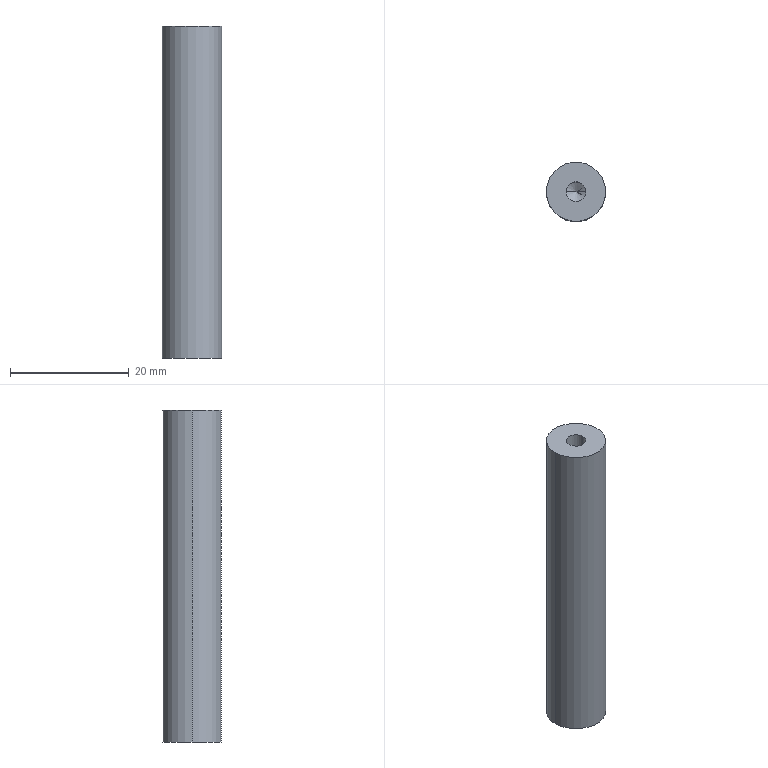Part | STEP file | 11-FG-Z00711 | 1 solid | 12 faces | box 10 x 10 x 56 mm | volume 4220 mm3 | cylinder 6 | cone 4 | plane 2 | commonest cylinder face diameters 3.3 x4 10 x2
STEP:
#1=CARTESIAN_POINT('',(1.65,0.,-45.9));
#2=VERTEX_POINT('',#1);
#3=CARTESIAN_POINT('',(-1.65,0.,-45.9));
#4=VERTEX_POINT('',#3);
#5=CARTESIAN_POINT('',(0.,0.,-45.9));
#6=DIRECTION('',(0.,0.,-1.));
#7=DIRECTION('',(-1.,0.,0.));
#8=AXIS2_PLACEMENT_3D('',#5,#6,#7);
#9=CIRCLE('',#8,1.65);
#10=EDGE_CURVE('',#2,#4,#9,.T.);
#11=ORIENTED_EDGE('',*,*,#10,.F.);
#12=CARTESIAN_POINT('',(1.65,0.,-56.));
#13=VERTEX_POINT('',#12);
#14=CARTESIAN_POINT('',(1.65,0.,-56.));
#15=DIRECTION('',(0.,0.,-1.));
#16=VECTOR('',#15,1000.);
#17=LINE('',#14,#16);
#18=EDGE_CURVE('',#2,#13,#17,.T.);
#19=ORIENTED_EDGE('',*,*,#18,.T.);
#20=CARTESIAN_POINT('',(-1.65,0.,-56.));
#21=VERTEX_POINT('',#20);
#22=CARTESIAN_POINT('',(0.,0.,-56.));
#23=DIRECTION('',(0.,0.,-1.));
#24=DIRECTION('',(-1.,0.,0.));
#25=AXIS2_PLACEMENT_3D('',#22,#23,#24);
#26=CIRCLE('',#25,1.65);
#27=EDGE_CURVE('',#13,#21,#26,.T.);
#28=ORIENTED_EDGE('',*,*,#27,.T.);
#29=CARTESIAN_POINT('',(-1.65,0.,-56.));
#30=DIRECTION('',(0.,0.,-1.));
#31=VECTOR('',#30,1000.);
#32=LINE('',#29,#31);
#33=EDGE_CURVE('',#4,#21,#32,.T.);
#34=ORIENTED_EDGE('',*,*,#33,.F.);
#35=EDGE_LOOP('',(#11,#19,#28,#34));
#36=FACE_OUTER_BOUND('',#35,.T.);
#37=CARTESIAN_POINT('',(0.,0.,-56.));
#38=DIRECTION('',(0.,0.,-1.));
#39=DIRECTION('',(-1.,0.,0.));
#40=AXIS2_PLACEMENT_3D('',#37,#38,#39);
#41=CYLINDRICAL_SURFACE('',#40,1.65);
#42=ADVANCED_FACE('',(#36),#41,.F.);
#43=CARTESIAN_POINT('',(0.,0.,-44.909));
#44=VERTEX_POINT('',#43);
#45=CARTESIAN_POINT('',(-1.65,0.,-45.9));
#46=DIRECTION('',(-0.8572,0.,-0.515));
#47=VECTOR('',#46,1000.);
#48=LINE('',#45,#47);
#49=EDGE_CURVE('',#44,#4,#48,.T.);
#50=ORIENTED_EDGE('',*,*,#49,.F.);
#51=CARTESIAN_POINT('',(1.65,0.,-45.9));
#52=DIRECTION('',(0.8572,0.,-0.515));
#53=VECTOR('',#52,1000.);
#54=LINE('',#51,#53);
#55=EDGE_CURVE('',#44,#2,#54,.T.);
#56=ORIENTED_EDGE('',*,*,#55,.T.);
#57=ORIENTED_EDGE('',*,*,#10,.T.);
#58=EDGE_LOOP('',(#50,#56,#57));
#59=FACE_OUTER_BOUND('',#58,.T.);
#60=CARTESIAN_POINT('',(0.,0.,-45.9));
#61=DIRECTION('',(0.,0.,-1.));
#62=DIRECTION('',(-1.,0.,0.));
#63=AXIS2_PLACEMENT_3D('',#60,#61,#62);
#64=CONICAL_SURFACE('',#63,1.65,1.03);
#65=ADVANCED_FACE('',(#59),#64,.F.);
#66=CARTESIAN_POINT('',(-1.65,0.,-10.1));
#67=VERTEX_POINT('',#66);
#68=CARTESIAN_POINT('',(1.65,0.,-10.1));
#69=VERTEX_POINT('',#68);
#70=CARTESIAN_POINT('',(0.,0.,-10.1));
#71=DIRECTION('',(0.,0.,1.));
#72=DIRECTION('',(1.,0.,0.));
#73=AXIS2_PLACEMENT_3D('',#70,#71,#72);
#74=CIRCLE('',#73,1.65);
#75=EDGE_CURVE('',#67,#69,#74,.T.);
#76=ORIENTED_EDGE('',*,*,#75,.F.);
#77=CARTESIAN_POINT('',(-1.65,0.,0.));
#78=VERTEX_POINT('',#77);
#79=CARTESIAN_POINT('',(-1.65,0.,0.));
#80=DIRECTION('',(0.,0.,1.));
#81=VECTOR('',#80,1000.);
#82=LINE('',#79,#81);
#83=EDGE_CURVE('',#67,#78,#82,.T.);
#84=ORIENTED_EDGE('',*,*,#83,.T.);
#85=CARTESIAN_POINT('',(1.65,0.,0.));
#86=VERTEX_POINT('',#85);
#87=CARTESIAN_POINT('',(0.,0.,0.));
#88=DIRECTION('',(0.,0.,1.));
#89=DIRECTION('',(1.,0.,0.));
#90=AXIS2_PLACEMENT_3D('',#87,#88,#89);
#91=CIRCLE('',#90,1.65);
#92=EDGE_CURVE('',#78,#86,#91,.T.);
#93=ORIENTED_EDGE('',*,*,#92,.T.);
#94=CARTESIAN_POINT('',(1.65,0.,0.));
#95=DIRECTION('',(0.,0.,1.));
#96=VECTOR('',#95,1000.);
#97=LINE('',#94,#96);
#98=EDGE_CURVE('',#69,#86,#97,.T.);
#99=ORIENTED_EDGE('',*,*,#98,.F.);
#100=EDGE_LOOP('',(#76,#84,#93,#99));
#101=FACE_OUTER_BOUND('',#100,.T.);
#102=CARTESIAN_POINT('',(0.,0.,0.));
#103=DIRECTION('',(0.,0.,1.));
#104=DIRECTION('',(1.,0.,0.));
#105=AXIS2_PLACEMENT_3D('',#102,#103,#104);
#106=CYLINDRICAL_SURFACE('',#105,1.65);
#107=ADVANCED_FACE('',(#101),#106,.F.);
#108=CARTESIAN_POINT('',(0.,0.,-11.091));
#109=VERTEX_POINT('',#108);
#110=CARTESIAN_POINT('',(1.65,0.,-10.1));
#111=DIRECTION('',(0.8572,0.,0.515));
#112=VECTOR('',#111,1000.);
#113=LINE('',#110,#112);
#114=EDGE_CURVE('',#109,#69,#113,.T.);
#115=ORIENTED_EDGE('',*,*,#114,.F.);
#116=CARTESIAN_POINT('',(-1.65,0.,-10.1));
#117=DIRECTION('',(-0.8572,0.,0.515));
#118=VECTOR('',#117,1000.);
#119=LINE('',#116,#118);
#120=EDGE_CURVE('',#109,#67,#119,.T.);
#121=ORIENTED_EDGE('',*,*,#120,.T.);
#122=ORIENTED_EDGE('',*,*,#75,.T.);
#123=EDGE_LOOP('',(#115,#121,#122));
#124=FACE_OUTER_BOUND('',#123,.T.);
#125=CARTESIAN_POINT('',(0.,0.,-10.1));
#126=DIRECTION('',(0.,0.,1.));
#127=DIRECTION('',(1.,0.,0.));
#128=AXIS2_PLACEMENT_3D('',#125,#126,#127);
#129=CONICAL_SURFACE('',#128,1.65,1.03);
#130=ADVANCED_FACE('',(#124),#129,.F.);
#131=CARTESIAN_POINT('',(5.,0.,-56.));
#132=VERTEX_POINT('',#131);
#133=CARTESIAN_POINT('',(-5.,0.,-56.));
#134=VERTEX_POINT('',#133);
#135=CARTESIAN_POINT('',(0.,0.,-56.));
#136=DIRECTION('',(0.,0.,1.));
#137=DIRECTION('',(1.,0.,0.));
#138=AXIS2_PLACEMENT_3D('',#135,#136,#137);
#139=CIRCLE('',#138,5.);
#140=EDGE_CURVE('',#132,#134,#139,.T.);
#141=ORIENTED_EDGE('',*,*,#140,.T.);
#142=CARTESIAN_POINT('',(-5.,0.,0.));
#143=VERTEX_POINT('',#142);
#144=CARTESIAN_POINT('',(-5.,0.,-56.));
#145=DIRECTION('',(0.,0.,1.));
#146=VECTOR('',#145,1000.);
#147=LINE('',#144,#146);
#148=EDGE_CURVE('',#134,#143,#147,.T.);
#149=ORIENTED_EDGE('',*,*,#148,.T.);
#150=CARTESIAN_POINT('',(5.,0.,0.));
#151=VERTEX_POINT('',#150);
#152=CARTESIAN_POINT('',(0.,0.,0.));
#153=DIRECTION('',(0.,0.,1.));
#154=DIRECTION('',(1.,0.,0.));
#155=AXIS2_PLACEMENT_3D('',#152,#153,#154);
#156=CIRCLE('',#155,5.);
#157=EDGE_CURVE('',#151,#143,#156,.T.);
#158=ORIENTED_EDGE('',*,*,#157,.F.);
#159=CARTESIAN_POINT('',(5.,0.,-56.));
#160=DIRECTION('',(0.,0.,1.));
#161=VECTOR('',#160,1000.);
#162=LINE('',#159,#161);
#163=EDGE_CURVE('',#132,#151,#162,.T.);
#164=ORIENTED_EDGE('',*,*,#163,.F.);
#165=EDGE_LOOP('',(#141,#149,#158,#164));
#166=FACE_OUTER_BOUND('',#165,.T.);
#167=CARTESIAN_POINT('',(0.,0.,-56.));
#168=DIRECTION('',(0.,0.,1.));
#169=DIRECTION('',(1.,0.,0.));
#170=AXIS2_PLACEMENT_3D('',#167,#168,#169);
#171=CYLINDRICAL_SURFACE('',#170,5.);
#172=ADVANCED_FACE('',(#166),#171,.T.);
#173=ORIENTED_EDGE('',*,*,#148,.F.);
#174=CARTESIAN_POINT('',(0.,0.,-56.));
#175=DIRECTION('',(0.,0.,1.));
#176=DIRECTION('',(1.,0.,0.));
#177=AXIS2_PLACEMENT_3D('',#174,#175,#176);
#178=CIRCLE('',#177,5.);
#179=EDGE_CURVE('',#134,#132,#178,.T.);
#180=ORIENTED_EDGE('',*,*,#179,.T.);
#181=ORIENTED_EDGE('',*,*,#163,.T.);
#182=CARTESIAN_POINT('',(0.,0.,0.));
#183=DIRECTION('',(0.,0.,1.));
#184=DIRECTION('',(1.,0.,0.));
#185=AXIS2_PLACEMENT_3D('',#182,#183,#184);
#186=CIRCLE('',#185,5.);
#187=EDGE_CURVE('',#143,#151,#186,.T.);
#188=ORIENTED_EDGE('',*,*,#187,.F.);
#189=EDGE_LOOP('',(#173,#180,#181,#188));
#190=FACE_OUTER_BOUND('',#189,.T.);
#191=CARTESIAN_POINT('',(0.,0.,-56.));
#192=DIRECTION('',(0.,0.,1.));
#193=DIRECTION('',(1.,0.,0.));
#194=AXIS2_PLACEMENT_3D('',#191,#192,#193);
#195=CYLINDRICAL_SURFACE('',#194,5.);
#196=ADVANCED_FACE('',(#190),#195,.T.);
#197=CARTESIAN_POINT('',(0.,0.,-56.));
#198=DIRECTION('',(0.,0.,-1.));
#199=DIRECTION('',(-1.,0.,0.));
#200=AXIS2_PLACEMENT_3D('',#197,#198,#199);
#201=CIRCLE('',#200,1.65);
#202=EDGE_CURVE('',#21,#13,#201,.T.);
#203=ORIENTED_EDGE('',*,*,#202,.F.);
#204=ORIENTED_EDGE('',*,*,#27,.F.);
#205=EDGE_LOOP('',(#203,#204));
#206=FACE_BOUND('',#205,.T.);
#207=ORIENTED_EDGE('',*,*,#140,.F.);
#208=ORIENTED_EDGE('',*,*,#179,.F.);
#209=EDGE_LOOP('',(#207,#208));
#210=FACE_OUTER_BOUND('',#209,.T.);
#211=CARTESIAN_POINT('',(0.,0.,-56.));
#212=DIRECTION('',(0.,0.,1.));
#213=DIRECTION('',(1.,0.,0.));
#214=AXIS2_PLACEMENT_3D('',#211,#212,#213);
#215=PLANE('',#214);
#216=ADVANCED_FACE('',(#206,#210),#215,.F.);
#217=CARTESIAN_POINT('',(0.,0.,0.));
#218=DIRECTION('',(0.,0.,1.));
#219=DIRECTION('',(1.,0.,0.));
#220=AXIS2_PLACEMENT_3D('',#217,#218,#219);
#221=CIRCLE('',#220,1.65);
#222=EDGE_CURVE('',#86,#78,#221,.T.);
#223=ORIENTED_EDGE('',*,*,#222,.F.);
#224=ORIENTED_EDGE('',*,*,#92,.F.);
#225=EDGE_LOOP('',(#223,#224));
#226=FACE_BOUND('',#225,.T.);
#227=ORIENTED_EDGE('',*,*,#157,.T.);
#228=ORIENTED_EDGE('',*,*,#187,.T.);
#229=EDGE_LOOP('',(#227,#228));
#230=FACE_OUTER_BOUND('',#229,.T.);
#231=CARTESIAN_POINT('',(0.,0.,0.));
#232=DIRECTION('',(0.,0.,1.));
#233=DIRECTION('',(1.,0.,0.));
#234=AXIS2_PLACEMENT_3D('',#231,#232,#233);
#235=PLANE('',#234);
#236=ADVANCED_FACE('',(#226,#230),#235,.T.);
#237=ORIENTED_EDGE('',*,*,#120,.F.);
#238=ORIENTED_EDGE('',*,*,#114,.T.);
#239=CARTESIAN_POINT('',(0.,0.,-10.1));
#240=DIRECTION('',(0.,0.,1.));
#241=DIRECTION('',(1.,0.,0.));
#242=AXIS2_PLACEMENT_3D('',#239,#240,#241);
#243=CIRCLE('',#242,1.65);
#244=EDGE_CURVE('',#69,#67,#243,.T.);
#245=ORIENTED_EDGE('',*,*,#244,.T.);
#246=EDGE_LOOP('',(#237,#238,#245));
#247=FACE_OUTER_BOUND('',#246,.T.);
#248=CARTESIAN_POINT('',(0.,0.,-10.1));
#249=DIRECTION('',(0.,0.,1.));
#250=DIRECTION('',(1.,0.,0.));
#251=AXIS2_PLACEMENT_3D('',#248,#249,#250);
#252=CONICAL_SURFACE('',#251,1.65,1.03);
#253=ADVANCED_FACE('',(#247),#252,.F.);
#254=ORIENTED_EDGE('',*,*,#83,.F.);
#255=ORIENTED_EDGE('',*,*,#244,.F.);
#256=ORIENTED_EDGE('',*,*,#98,.T.);
#257=ORIENTED_EDGE('',*,*,#222,.T.);
#258=EDGE_LOOP('',(#254,#255,#256,#257));
#259=FACE_OUTER_BOUND('',#258,.T.);
#260=CARTESIAN_POINT('',(0.,0.,0.));
#261=DIRECTION('',(0.,0.,1.));
#262=DIRECTION('',(1.,0.,0.));
#263=AXIS2_PLACEMENT_3D('',#260,#261,#262);
#264=CYLINDRICAL_SURFACE('',#263,1.65);
#265=ADVANCED_FACE('',(#259),#264,.F.);
#266=ORIENTED_EDGE('',*,*,#55,.F.);
#267=ORIENTED_EDGE('',*,*,#49,.T.);
#268=CARTESIAN_POINT('',(0.,0.,-45.9));
#269=DIRECTION('',(0.,0.,-1.));
#270=DIRECTION('',(-1.,0.,0.));
#271=AXIS2_PLACEMENT_3D('',#268,#269,#270);
#272=CIRCLE('',#271,1.65);
#273=EDGE_CURVE('',#4,#2,#272,.T.);
#274=ORIENTED_EDGE('',*,*,#273,.T.);
#275=EDGE_LOOP('',(#266,#267,#274));
#276=FACE_OUTER_BOUND('',#275,.T.);
#277=CARTESIAN_POINT('',(0.,0.,-45.9));
#278=DIRECTION('',(0.,0.,-1.));
#279=DIRECTION('',(-1.,0.,0.));
#280=AXIS2_PLACEMENT_3D('',#277,#278,#279);
#281=CONICAL_SURFACE('',#280,1.65,1.03);
#282=ADVANCED_FACE('',(#276),#281,.F.);
#283=ORIENTED_EDGE('',*,*,#18,.F.);
#284=ORIENTED_EDGE('',*,*,#273,.F.);
#285=ORIENTED_EDGE('',*,*,#33,.T.);
#286=ORIENTED_EDGE('',*,*,#202,.T.);
#287=EDGE_LOOP('',(#283,#284,#285,#286));
#288=FACE_OUTER_BOUND('',#287,.T.);
#289=CARTESIAN_POINT('',(0.,0.,-56.));
#290=DIRECTION('',(0.,0.,-1.));
#291=DIRECTION('',(-1.,0.,0.));
#292=AXIS2_PLACEMENT_3D('',#289,#290,#291);
#293=CYLINDRICAL_SURFACE('',#292,1.65);
#294=ADVANCED_FACE('',(#288),#293,.F.);
#295=CLOSED_SHELL('',(#42,#65,#107,#130,#172,#196,#216,#236,#253,#265,#282,#294));
#296=MANIFOLD_SOLID_BREP('',#295);
#297=CARTESIAN_POINT('',(0.,0.,0.));
#298=DIRECTION('',(0.,0.,1.));
#299=DIRECTION('',(1.,0.,0.));
#300=AXIS2_PLACEMENT_3D('',#297,#298,#299);
#301=(LENGTH_UNIT()NAMED_UNIT(*)SI_UNIT(.MILLI.,.METRE.));
#302=UNCERTAINTY_MEASURE_WITH_UNIT(LENGTH_MEASURE(0.00001),#301,'','');
#303=(NAMED_UNIT(*)PLANE_ANGLE_UNIT()SI_UNIT($,.RADIAN.));
#304=(NAMED_UNIT(*)SI_UNIT($,.STERADIAN.)SOLID_ANGLE_UNIT());
#305=(GEOMETRIC_REPRESENTATION_CONTEXT(3)GLOBAL_UNCERTAINTY_ASSIGNED_CONTEXT((#302))GLOBAL_UNIT_ASSIGNED_CONTEXT((#301,#303,#304))REPRESENTATION_CONTEXT('',''));
#306=ADVANCED_BREP_SHAPE_REPRESENTATION('',(#296,#300),#305);